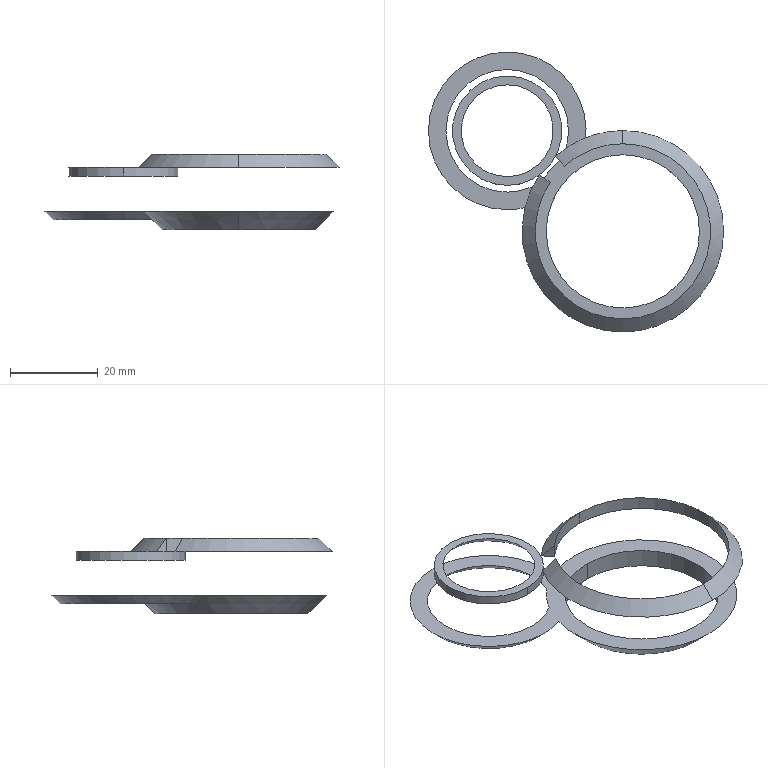Part | SolidWorks | features BaseBody 3 | 3 solids | 25 faces | box 67.409 x 63.969 x 17.243 mm | volume 2142 mm3 | cone 13 | cylinder 7 | plane 5 | commonest cylinder face diameters 40 x3 25 x2 35 x2
STEP:
#1=CARTESIAN_POINT('',(128.912,61.709,-226.962));
#2=VERTEX_POINT('',#1);
#3=CARTESIAN_POINT('',(128.912,96.709,-226.962));
#4=VERTEX_POINT('',#3);
#5=CARTESIAN_POINT('',(128.912,79.209,-226.962));
#6=DIRECTION('',(0.,0.,-1.));
#7=DIRECTION('',(0.,1.,0.));
#8=AXIS2_PLACEMENT_3D('',#5,#6,#7);
#9=CIRCLE('',#8,17.5);
#10=EDGE_CURVE('',#2,#4,#9,.T.);
#11=ORIENTED_EDGE('',*,*,#10,.F.);
#12=CARTESIAN_POINT('',(128.912,61.709,-231.204));
#13=VERTEX_POINT('',#12);
#14=CARTESIAN_POINT('',(128.912,61.709,-232.962));
#15=DIRECTION('',(0.,0.,-1.));
#16=VECTOR('',#15,1000.);
#17=LINE('',#14,#16);
#18=EDGE_CURVE('',#2,#13,#17,.T.);
#19=ORIENTED_EDGE('',*,*,#18,.T.);
#20=CARTESIAN_POINT('',(128.912,96.709,-231.204));
#21=VERTEX_POINT('',#20);
#22=CARTESIAN_POINT('',(128.912,79.209,-231.204));
#23=DIRECTION('',(0.,0.,1.));
#24=DIRECTION('',(0.,1.,0.));
#25=AXIS2_PLACEMENT_3D('',#22,#23,#24);
#26=CIRCLE('',#25,17.5);
#27=EDGE_CURVE('',#21,#13,#26,.T.);
#28=ORIENTED_EDGE('',*,*,#27,.F.);
#29=CARTESIAN_POINT('',(128.912,96.709,-232.962));
#30=DIRECTION('',(0.,0.,-1.));
#31=VECTOR('',#30,1000.);
#32=LINE('',#29,#31);
#33=EDGE_CURVE('',#4,#21,#32,.T.);
#34=ORIENTED_EDGE('',*,*,#33,.F.);
#35=EDGE_LOOP('',(#11,#19,#28,#34));
#36=FACE_OUTER_BOUND('',#35,.T.);
#37=CARTESIAN_POINT('',(128.912,79.209,-232.962));
#38=DIRECTION('',(0.,0.,-1.));
#39=DIRECTION('',(0.,1.,0.));
#40=AXIS2_PLACEMENT_3D('',#37,#38,#39);
#41=CYLINDRICAL_SURFACE('',#40,17.5);
#42=ADVANCED_FACE('',(#36),#41,.F.);
#43=CARTESIAN_POINT('',(102.503,88.178,-226.962));
#44=VERTEX_POINT('',#43);
#45=CARTESIAN_POINT('',(102.503,116.178,-226.962));
#46=VERTEX_POINT('',#45);
#47=CARTESIAN_POINT('',(102.503,102.178,-226.962));
#48=DIRECTION('',(0.,0.,-1.));
#49=DIRECTION('',(0.,1.,0.));
#50=AXIS2_PLACEMENT_3D('',#47,#48,#49);
#51=CIRCLE('',#50,14.);
#52=EDGE_CURVE('',#44,#46,#51,.T.);
#53=ORIENTED_EDGE('',*,*,#52,.F.);
#54=CARTESIAN_POINT('',(102.503,86.178,-228.962));
#55=VERTEX_POINT('',#54);
#56=CARTESIAN_POINT('',(102.503,86.178,-228.962));
#57=DIRECTION('',(0.,-0.7071,-0.7071));
#58=VECTOR('',#57,1000.);
#59=LINE('',#56,#58);
#60=EDGE_CURVE('',#44,#55,#59,.T.);
#61=ORIENTED_EDGE('',*,*,#60,.T.);
#62=CARTESIAN_POINT('',(102.503,118.178,-228.962));
#63=VERTEX_POINT('',#62);
#64=CARTESIAN_POINT('',(102.503,102.178,-228.962));
#65=DIRECTION('',(0.,0.,1.));
#66=DIRECTION('',(0.7855,0.6189,0.));
#67=AXIS2_PLACEMENT_3D('',#64,#65,#66);
#68=CIRCLE('',#67,16.);
#69=EDGE_CURVE('',#63,#55,#68,.T.);
#70=ORIENTED_EDGE('',*,*,#69,.F.);
#71=CARTESIAN_POINT('',(102.503,118.178,-228.962));
#72=DIRECTION('',(0.,0.7071,-0.7071));
#73=VECTOR('',#72,1000.);
#74=LINE('',#71,#73);
#75=EDGE_CURVE('',#46,#63,#74,.T.);
#76=ORIENTED_EDGE('',*,*,#75,.F.);
#77=EDGE_LOOP('',(#53,#61,#70,#76));
#78=FACE_OUTER_BOUND('',#77,.T.);
#79=CARTESIAN_POINT('',(102.503,102.178,-228.962));
#80=DIRECTION('',(0.,0.,-1.));
#81=DIRECTION('',(0.,1.,0.));
#82=AXIS2_PLACEMENT_3D('',#79,#80,#81);
#83=CONICAL_SURFACE('',#82,16.,0.7854);
#84=ADVANCED_FACE('',(#78),#83,.F.);
#85=CARTESIAN_POINT('',(115.043,95.955,-226.962));
#86=VERTEX_POINT('',#85);
#87=CARTESIAN_POINT('',(102.503,102.178,-226.962));
#88=DIRECTION('',(0.,0.,-1.));
#89=DIRECTION('',(0.,1.,0.));
#90=AXIS2_PLACEMENT_3D('',#87,#88,#89);
#91=CIRCLE('',#90,14.);
#92=EDGE_CURVE('',#46,#86,#91,.T.);
#93=ORIENTED_EDGE('',*,*,#92,.F.);
#94=ORIENTED_EDGE('',*,*,#75,.T.);
#95=CARTESIAN_POINT('',(116.63,94.667,-228.962));
#96=VERTEX_POINT('',#95);
#97=CARTESIAN_POINT('',(102.503,102.178,-228.962));
#98=DIRECTION('',(0.,0.,1.));
#99=DIRECTION('',(0.7855,0.6189,0.));
#100=AXIS2_PLACEMENT_3D('',#97,#98,#99);
#101=CIRCLE('',#100,16.);
#102=EDGE_CURVE('',#96,#63,#101,.T.);
#103=ORIENTED_EDGE('',*,*,#102,.F.);
#104=CARTESIAN_POINT('',(115.043,95.955,-226.962));
#105=CARTESIAN_POINT('',(115.578,95.532,-227.628));
#106=CARTESIAN_POINT('',(116.106,95.102,-228.295));
#107=CARTESIAN_POINT('',(116.63,94.667,-228.962));
#108=B_SPLINE_CURVE_WITH_KNOTS('',3,(#104,#105,#106,#107),.UNSPECIFIED.,.F.,.F.,(4,4),(0.,0.002859),.UNSPECIFIED.);
#109=EDGE_CURVE('',#86,#96,#108,.T.);
#110=ORIENTED_EDGE('',*,*,#109,.F.);
#111=EDGE_LOOP('',(#93,#94,#103,#110));
#112=FACE_OUTER_BOUND('',#111,.T.);
#113=CARTESIAN_POINT('',(102.503,102.178,-228.962));
#114=DIRECTION('',(0.,0.,-1.));
#115=DIRECTION('',(0.,1.,0.));
#116=AXIS2_PLACEMENT_3D('',#113,#114,#115);
#117=CONICAL_SURFACE('',#116,16.,0.7854);
#118=ADVANCED_FACE('',(#112),#117,.F.);
#119=CARTESIAN_POINT('',(128.912,79.209,-231.204));
#120=DIRECTION('',(0.,0.,1.));
#121=DIRECTION('',(0.,1.,0.));
#122=AXIS2_PLACEMENT_3D('',#119,#120,#121);
#123=CIRCLE('',#122,17.5);
#124=EDGE_CURVE('',#13,#21,#123,.T.);
#125=ORIENTED_EDGE('',*,*,#124,.T.);
#126=CARTESIAN_POINT('',(128.912,100.952,-226.962));
#127=VERTEX_POINT('',#126);
#128=CARTESIAN_POINT('',(128.912,100.952,-226.962));
#129=DIRECTION('',(0.,0.7071,0.7071));
#130=VECTOR('',#129,1000.);
#131=LINE('',#128,#130);
#132=EDGE_CURVE('',#21,#127,#131,.T.);
#133=ORIENTED_EDGE('',*,*,#132,.T.);
#134=CARTESIAN_POINT('',(128.912,57.467,-226.962));
#135=VERTEX_POINT('',#134);
#136=CARTESIAN_POINT('',(128.912,79.209,-226.962));
#137=DIRECTION('',(0.,0.,1.));
#138=DIRECTION('',(0.,-1.,0.));
#139=AXIS2_PLACEMENT_3D('',#136,#137,#138);
#140=CIRCLE('',#139,21.743);
#141=EDGE_CURVE('',#135,#127,#140,.T.);
#142=ORIENTED_EDGE('',*,*,#141,.F.);
#143=CARTESIAN_POINT('',(128.912,57.467,-226.962));
#144=DIRECTION('',(0.,-0.7071,0.7071));
#145=VECTOR('',#144,1000.);
#146=LINE('',#143,#145);
#147=EDGE_CURVE('',#13,#135,#146,.T.);
#148=ORIENTED_EDGE('',*,*,#147,.F.);
#149=EDGE_LOOP('',(#125,#133,#142,#148));
#150=FACE_OUTER_BOUND('',#149,.T.);
#151=CARTESIAN_POINT('',(128.912,79.209,-226.962));
#152=DIRECTION('',(0.,0.,1.));
#153=DIRECTION('',(0.,-1.,0.));
#154=AXIS2_PLACEMENT_3D('',#151,#152,#153);
#155=CONICAL_SURFACE('',#154,21.743,0.7854);
#156=ADVANCED_FACE('',(#150),#155,.T.);
#157=ORIENTED_EDGE('',*,*,#102,.T.);
#158=CARTESIAN_POINT('',(102.503,120.178,-226.962));
#159=VERTEX_POINT('',#158);
#160=CARTESIAN_POINT('',(102.503,120.178,-226.962));
#161=DIRECTION('',(0.,0.7071,0.7071));
#162=VECTOR('',#161,1000.);
#163=LINE('',#160,#162);
#164=EDGE_CURVE('',#63,#159,#163,.T.);
#165=ORIENTED_EDGE('',*,*,#164,.T.);
#166=CARTESIAN_POINT('',(120.246,99.151,-226.962));
#167=VERTEX_POINT('',#166);
#168=CARTESIAN_POINT('',(102.503,102.178,-226.962));
#169=DIRECTION('',(0.,0.,1.));
#170=DIRECTION('',(0.,-1.,0.));
#171=AXIS2_PLACEMENT_3D('',#168,#169,#170);
#172=CIRCLE('',#171,18.);
#173=EDGE_CURVE('',#167,#159,#172,.T.);
#174=ORIENTED_EDGE('',*,*,#173,.F.);
#175=CARTESIAN_POINT('',(116.63,94.667,-228.962));
#176=CARTESIAN_POINT('',(117.273,95.439,-228.757));
#177=CARTESIAN_POINT('',(117.891,96.196,-228.476));
#178=CARTESIAN_POINT('',(119.093,97.689,-227.798));
#179=CARTESIAN_POINT('',(119.676,98.424,-227.401));
#180=CARTESIAN_POINT('',(120.246,99.151,-226.962));
#181=B_SPLINE_CURVE_WITH_KNOTS('',3,(#175,#176,#177,#178,#179,#180),.UNSPECIFIED.,.F.,.F.,(4,2,4),(0.,0.003049,0.006098),.UNSPECIFIED.);
#182=EDGE_CURVE('',#96,#167,#181,.T.);
#183=ORIENTED_EDGE('',*,*,#182,.F.);
#184=EDGE_LOOP('',(#157,#165,#174,#183));
#185=FACE_OUTER_BOUND('',#184,.T.);
#186=CARTESIAN_POINT('',(102.503,102.178,-226.962));
#187=DIRECTION('',(0.,0.,1.));
#188=DIRECTION('',(0.,-1.,0.));
#189=AXIS2_PLACEMENT_3D('',#186,#187,#188);
#190=CONICAL_SURFACE('',#189,18.,0.7854);
#191=ADVANCED_FACE('',(#185),#190,.T.);
#192=ORIENTED_EDGE('',*,*,#164,.F.);
#193=ORIENTED_EDGE('',*,*,#69,.T.);
#194=CARTESIAN_POINT('',(102.503,84.178,-226.962));
#195=VERTEX_POINT('',#194);
#196=CARTESIAN_POINT('',(102.503,84.178,-226.962));
#197=DIRECTION('',(0.,-0.7071,0.7071));
#198=VECTOR('',#197,1000.);
#199=LINE('',#196,#198);
#200=EDGE_CURVE('',#55,#195,#199,.T.);
#201=ORIENTED_EDGE('',*,*,#200,.T.);
#202=CARTESIAN_POINT('',(102.503,102.178,-226.962));
#203=DIRECTION('',(0.,0.,1.));
#204=DIRECTION('',(0.,-1.,0.));
#205=AXIS2_PLACEMENT_3D('',#202,#203,#204);
#206=CIRCLE('',#205,18.);
#207=EDGE_CURVE('',#159,#195,#206,.T.);
#208=ORIENTED_EDGE('',*,*,#207,.F.);
#209=EDGE_LOOP('',(#192,#193,#201,#208));
#210=FACE_OUTER_BOUND('',#209,.T.);
#211=CARTESIAN_POINT('',(102.503,102.178,-226.962));
#212=DIRECTION('',(0.,0.,1.));
#213=DIRECTION('',(0.,-1.,0.));
#214=AXIS2_PLACEMENT_3D('',#211,#212,#213);
#215=CONICAL_SURFACE('',#214,18.,0.7854);
#216=ADVANCED_FACE('',(#210),#215,.T.);
#217=CARTESIAN_POINT('',(128.912,79.209,-226.962));
#218=DIRECTION('',(0.,0.,-1.));
#219=DIRECTION('',(0.,1.,0.));
#220=AXIS2_PLACEMENT_3D('',#217,#218,#219);
#221=CIRCLE('',#220,17.5);
#222=EDGE_CURVE('',#4,#2,#221,.T.);
#223=ORIENTED_EDGE('',*,*,#222,.T.);
#224=ORIENTED_EDGE('',*,*,#10,.T.);
#225=EDGE_LOOP('',(#223,#224));
#226=FACE_BOUND('',#225,.T.);
#227=CARTESIAN_POINT('',(110.405,90.621,-226.962));
#228=VERTEX_POINT('',#227);
#229=CARTESIAN_POINT('',(128.912,79.209,-226.962));
#230=DIRECTION('',(0.,0.,1.));
#231=DIRECTION('',(0.,-1.,0.));
#232=AXIS2_PLACEMENT_3D('',#229,#230,#231);
#233=CIRCLE('',#232,21.743);
#234=EDGE_CURVE('',#86,#228,#233,.T.);
#235=ORIENTED_EDGE('',*,*,#234,.T.);
#236=CARTESIAN_POINT('',(102.503,102.178,-226.962));
#237=DIRECTION('',(0.,0.,-1.));
#238=DIRECTION('',(0.,1.,0.));
#239=AXIS2_PLACEMENT_3D('',#236,#237,#238);
#240=CIRCLE('',#239,14.);
#241=EDGE_CURVE('',#228,#44,#240,.T.);
#242=ORIENTED_EDGE('',*,*,#241,.T.);
#243=ORIENTED_EDGE('',*,*,#52,.T.);
#244=ORIENTED_EDGE('',*,*,#92,.T.);
#245=EDGE_LOOP('',(#235,#242,#243,#244));
#246=FACE_BOUND('',#245,.T.);
#247=ORIENTED_EDGE('',*,*,#173,.T.);
#248=ORIENTED_EDGE('',*,*,#207,.T.);
#249=CARTESIAN_POINT('',(107.961,85.026,-226.962));
#250=VERTEX_POINT('',#249);
#251=CARTESIAN_POINT('',(102.503,102.178,-226.962));
#252=DIRECTION('',(0.,0.,1.));
#253=DIRECTION('',(0.,-1.,0.));
#254=AXIS2_PLACEMENT_3D('',#251,#252,#253);
#255=CIRCLE('',#254,18.);
#256=EDGE_CURVE('',#195,#250,#255,.T.);
#257=ORIENTED_EDGE('',*,*,#256,.T.);
#258=CARTESIAN_POINT('',(128.912,79.209,-226.962));
#259=DIRECTION('',(0.,0.,1.));
#260=DIRECTION('',(0.,-1.,0.));
#261=AXIS2_PLACEMENT_3D('',#258,#259,#260);
#262=CIRCLE('',#261,21.743);
#263=EDGE_CURVE('',#250,#135,#262,.T.);
#264=ORIENTED_EDGE('',*,*,#263,.T.);
#265=ORIENTED_EDGE('',*,*,#141,.T.);
#266=CARTESIAN_POINT('',(128.912,79.209,-226.962));
#267=DIRECTION('',(0.,0.,1.));
#268=DIRECTION('',(0.,-1.,0.));
#269=AXIS2_PLACEMENT_3D('',#266,#267,#268);
#270=CIRCLE('',#269,21.743);
#271=EDGE_CURVE('',#127,#167,#270,.T.);
#272=ORIENTED_EDGE('',*,*,#271,.T.);
#273=EDGE_LOOP('',(#247,#248,#257,#264,#265,#272));
#274=FACE_OUTER_BOUND('',#273,.T.);
#275=CARTESIAN_POINT('',(115.707,90.694,-226.962));
#276=DIRECTION('',(0.,0.,1.));
#277=DIRECTION('',(0.,-1.,0.));
#278=AXIS2_PLACEMENT_3D('',#275,#276,#277);
#279=PLANE('',#278);
#280=ADVANCED_FACE('',(#226,#246,#274),#279,.T.);
#281=ORIENTED_EDGE('',*,*,#18,.F.);
#282=ORIENTED_EDGE('',*,*,#222,.F.);
#283=ORIENTED_EDGE('',*,*,#33,.T.);
#284=ORIENTED_EDGE('',*,*,#124,.F.);
#285=EDGE_LOOP('',(#281,#282,#283,#284));
#286=FACE_OUTER_BOUND('',#285,.T.);
#287=CARTESIAN_POINT('',(128.912,79.209,-232.962));
#288=DIRECTION('',(0.,0.,-1.));
#289=DIRECTION('',(0.,1.,0.));
#290=AXIS2_PLACEMENT_3D('',#287,#288,#289);
#291=CYLINDRICAL_SURFACE('',#290,17.5);
#292=ADVANCED_FACE('',(#286),#291,.F.);
#293=ORIENTED_EDGE('',*,*,#60,.F.);
#294=ORIENTED_EDGE('',*,*,#241,.F.);
#295=CARTESIAN_POINT('',(111.901,89.229,-228.962));
#296=VERTEX_POINT('',#295);
#297=CARTESIAN_POINT('',(111.901,89.229,-228.962));
#298=CARTESIAN_POINT('',(111.396,89.687,-228.295));
#299=CARTESIAN_POINT('',(110.898,90.151,-227.628));
#300=CARTESIAN_POINT('',(110.405,90.621,-226.962));
#301=B_SPLINE_CURVE_WITH_KNOTS('',3,(#297,#298,#299,#300),.UNSPECIFIED.,.F.,.F.,(4,4),(0.,0.002859),.UNSPECIFIED.);
#302=EDGE_CURVE('',#296,#228,#301,.T.);
#303=ORIENTED_EDGE('',*,*,#302,.F.);
#304=CARTESIAN_POINT('',(102.503,102.178,-228.962));
#305=DIRECTION('',(0.,0.,1.));
#306=DIRECTION('',(0.7855,0.6189,0.));
#307=AXIS2_PLACEMENT_3D('',#304,#305,#306);
#308=CIRCLE('',#307,16.);
#309=EDGE_CURVE('',#55,#296,#308,.T.);
#310=ORIENTED_EDGE('',*,*,#309,.F.);
#311=EDGE_LOOP('',(#293,#294,#303,#310));
#312=FACE_OUTER_BOUND('',#311,.T.);
#313=CARTESIAN_POINT('',(102.503,102.178,-228.962));
#314=DIRECTION('',(0.,0.,-1.));
#315=DIRECTION('',(0.,1.,0.));
#316=AXIS2_PLACEMENT_3D('',#313,#314,#315);
#317=CONICAL_SURFACE('',#316,16.,0.7854);
#318=ADVANCED_FACE('',(#312),#317,.F.);
#319=ORIENTED_EDGE('',*,*,#132,.F.);
#320=ORIENTED_EDGE('',*,*,#27,.T.);
#321=ORIENTED_EDGE('',*,*,#147,.T.);
#322=ORIENTED_EDGE('',*,*,#263,.F.);
#323=CARTESIAN_POINT('',(107.961,85.026,-226.962));
#324=CARTESIAN_POINT('',(108.602,85.691,-227.401));
#325=CARTESIAN_POINT('',(109.249,86.37,-227.798));
#326=CARTESIAN_POINT('',(110.56,87.767,-228.476));
#327=CARTESIAN_POINT('',(111.225,88.485,-228.757));
#328=CARTESIAN_POINT('',(111.901,89.229,-228.962));
#329=B_SPLINE_CURVE_WITH_KNOTS('',3,(#323,#324,#325,#326,#327,#328),.UNSPECIFIED.,.F.,.F.,(4,2,4),(0.,0.003049,0.006098),.UNSPECIFIED.);
#330=EDGE_CURVE('',#250,#296,#329,.T.);
#331=ORIENTED_EDGE('',*,*,#330,.T.);
#332=ORIENTED_EDGE('',*,*,#302,.T.);
#333=ORIENTED_EDGE('',*,*,#234,.F.);
#334=ORIENTED_EDGE('',*,*,#109,.T.);
#335=ORIENTED_EDGE('',*,*,#182,.T.);
#336=ORIENTED_EDGE('',*,*,#271,.F.);
#337=EDGE_LOOP('',(#319,#320,#321,#322,#331,#332,#333,#334,#335,#336));
#338=FACE_OUTER_BOUND('',#337,.T.);
#339=CARTESIAN_POINT('',(128.912,79.209,-226.962));
#340=DIRECTION('',(0.,0.,1.));
#341=DIRECTION('',(0.,-1.,0.));
#342=AXIS2_PLACEMENT_3D('',#339,#340,#341);
#343=CONICAL_SURFACE('',#342,21.743,0.7854);
#344=ADVANCED_FACE('',(#338),#343,.T.);
#345=ORIENTED_EDGE('',*,*,#200,.F.);
#346=ORIENTED_EDGE('',*,*,#309,.T.);
#347=ORIENTED_EDGE('',*,*,#330,.F.);
#348=ORIENTED_EDGE('',*,*,#256,.F.);
#349=EDGE_LOOP('',(#345,#346,#347,#348));
#350=FACE_OUTER_BOUND('',#349,.T.);
#351=CARTESIAN_POINT('',(102.503,102.178,-226.962));
#352=DIRECTION('',(0.,0.,1.));
#353=DIRECTION('',(0.,-1.,0.));
#354=AXIS2_PLACEMENT_3D('',#351,#352,#353);
#355=CONICAL_SURFACE('',#354,18.,0.7854);
#356=ADVANCED_FACE('',(#350),#355,.T.);
#357=CLOSED_SHELL('',(#42,#84,#118,#156,#191,#216,#280,#292,#318,#344,#356));
#358=MANIFOLD_SOLID_BREP('',#357);
#359=CARTESIAN_POINT('',(102.503,91.678,-216.962));
#360=VERTEX_POINT('',#359);
#361=CARTESIAN_POINT('',(102.503,112.678,-216.962));
#362=VERTEX_POINT('',#361);
#363=CARTESIAN_POINT('',(102.503,102.178,-216.962));
#364=DIRECTION('',(0.,0.,-1.));
#365=DIRECTION('',(0.,1.,0.));
#366=AXIS2_PLACEMENT_3D('',#363,#364,#365);
#367=CIRCLE('',#366,10.5);
#368=EDGE_CURVE('',#360,#362,#367,.T.);
#369=ORIENTED_EDGE('',*,*,#368,.F.);
#370=CARTESIAN_POINT('',(102.503,89.678,-218.962));
#371=VERTEX_POINT('',#370);
#372=CARTESIAN_POINT('',(102.503,89.678,-218.962));
#373=DIRECTION('',(0.,-0.7071,-0.7071));
#374=VECTOR('',#373,1000.);
#375=LINE('',#372,#374);
#376=EDGE_CURVE('',#360,#371,#375,.T.);
#377=ORIENTED_EDGE('',*,*,#376,.T.);
#378=CARTESIAN_POINT('',(102.503,114.678,-218.962));
#379=VERTEX_POINT('',#378);
#380=CARTESIAN_POINT('',(102.503,102.178,-218.962));
#381=DIRECTION('',(0.,0.,1.));
#382=DIRECTION('',(0.7855,0.6189,0.));
#383=AXIS2_PLACEMENT_3D('',#380,#381,#382);
#384=CIRCLE('',#383,12.5);
#385=EDGE_CURVE('',#379,#371,#384,.T.);
#386=ORIENTED_EDGE('',*,*,#385,.F.);
#387=CARTESIAN_POINT('',(102.503,114.678,-218.962));
#388=DIRECTION('',(0.,0.7071,-0.7071));
#389=VECTOR('',#388,1000.);
#390=LINE('',#387,#389);
#391=EDGE_CURVE('',#362,#379,#390,.T.);
#392=ORIENTED_EDGE('',*,*,#391,.F.);
#393=EDGE_LOOP('',(#369,#377,#386,#392));
#394=FACE_OUTER_BOUND('',#393,.T.);
#395=CARTESIAN_POINT('',(102.503,102.178,-218.962));
#396=DIRECTION('',(0.,0.,-1.));
#397=DIRECTION('',(0.,1.,0.));
#398=AXIS2_PLACEMENT_3D('',#395,#396,#397);
#399=CONICAL_SURFACE('',#398,12.5,0.7854);
#400=ADVANCED_FACE('',(#394),#399,.F.);
#401=CARTESIAN_POINT('',(102.503,102.178,-218.962));
#402=DIRECTION('',(0.,0.,1.));
#403=DIRECTION('',(0.7855,0.6189,0.));
#404=AXIS2_PLACEMENT_3D('',#401,#402,#403);
#405=CIRCLE('',#404,12.5);
#406=EDGE_CURVE('',#371,#379,#405,.T.);
#407=ORIENTED_EDGE('',*,*,#406,.T.);
#408=CARTESIAN_POINT('',(102.503,114.678,-216.962));
#409=VERTEX_POINT('',#408);
#410=CARTESIAN_POINT('',(102.503,114.678,-226.962));
#411=DIRECTION('',(0.,0.,1.));
#412=VECTOR('',#411,1000.);
#413=LINE('',#410,#412);
#414=EDGE_CURVE('',#379,#409,#413,.T.);
#415=ORIENTED_EDGE('',*,*,#414,.T.);
#416=CARTESIAN_POINT('',(102.503,89.678,-216.962));
#417=VERTEX_POINT('',#416);
#418=CARTESIAN_POINT('',(102.503,102.178,-216.962));
#419=DIRECTION('',(0.,0.,-1.));
#420=DIRECTION('',(0.,-1.,0.));
#421=AXIS2_PLACEMENT_3D('',#418,#419,#420);
#422=CIRCLE('',#421,12.5);
#423=EDGE_CURVE('',#409,#417,#422,.T.);
#424=ORIENTED_EDGE('',*,*,#423,.T.);
#425=CARTESIAN_POINT('',(102.503,89.678,-226.962));
#426=DIRECTION('',(0.,0.,1.));
#427=VECTOR('',#426,1000.);
#428=LINE('',#425,#427);
#429=EDGE_CURVE('',#371,#417,#428,.T.);
#430=ORIENTED_EDGE('',*,*,#429,.F.);
#431=EDGE_LOOP('',(#407,#415,#424,#430));
#432=FACE_OUTER_BOUND('',#431,.T.);
#433=CARTESIAN_POINT('',(102.503,102.178,-226.962));
#434=DIRECTION('',(0.,0.,1.));
#435=DIRECTION('',(0.,-1.,0.));
#436=AXIS2_PLACEMENT_3D('',#433,#434,#435);
#437=CYLINDRICAL_SURFACE('',#436,12.5);
#438=ADVANCED_FACE('',(#432),#437,.T.);
#439=ORIENTED_EDGE('',*,*,#376,.F.);
#440=CARTESIAN_POINT('',(102.503,102.178,-216.962));
#441=DIRECTION('',(0.,0.,-1.));
#442=DIRECTION('',(0.,1.,0.));
#443=AXIS2_PLACEMENT_3D('',#440,#441,#442);
#444=CIRCLE('',#443,10.5);
#445=EDGE_CURVE('',#362,#360,#444,.T.);
#446=ORIENTED_EDGE('',*,*,#445,.F.);
#447=ORIENTED_EDGE('',*,*,#391,.T.);
#448=ORIENTED_EDGE('',*,*,#406,.F.);
#449=EDGE_LOOP('',(#439,#446,#447,#448));
#450=FACE_OUTER_BOUND('',#449,.T.);
#451=CARTESIAN_POINT('',(102.503,102.178,-218.962));
#452=DIRECTION('',(0.,0.,-1.));
#453=DIRECTION('',(0.,1.,0.));
#454=AXIS2_PLACEMENT_3D('',#451,#452,#453);
#455=CONICAL_SURFACE('',#454,12.5,0.7854);
#456=ADVANCED_FACE('',(#450),#455,.F.);
#457=ORIENTED_EDGE('',*,*,#414,.F.);
#458=ORIENTED_EDGE('',*,*,#385,.T.);
#459=ORIENTED_EDGE('',*,*,#429,.T.);
#460=CARTESIAN_POINT('',(102.503,102.178,-216.962));
#461=DIRECTION('',(0.,0.,-1.));
#462=DIRECTION('',(0.,-1.,0.));
#463=AXIS2_PLACEMENT_3D('',#460,#461,#462);
#464=CIRCLE('',#463,12.5);
#465=EDGE_CURVE('',#417,#409,#464,.T.);
#466=ORIENTED_EDGE('',*,*,#465,.T.);
#467=EDGE_LOOP('',(#457,#458,#459,#466));
#468=FACE_OUTER_BOUND('',#467,.T.);
#469=CARTESIAN_POINT('',(102.503,102.178,-226.962));
#470=DIRECTION('',(0.,0.,1.));
#471=DIRECTION('',(0.,-1.,0.));
#472=AXIS2_PLACEMENT_3D('',#469,#470,#471);
#473=CYLINDRICAL_SURFACE('',#472,12.5);
#474=ADVANCED_FACE('',(#468),#473,.T.);
#475=ORIENTED_EDGE('',*,*,#445,.T.);
#476=ORIENTED_EDGE('',*,*,#368,.T.);
#477=EDGE_LOOP('',(#475,#476));
#478=FACE_BOUND('',#477,.T.);
#479=ORIENTED_EDGE('',*,*,#465,.F.);
#480=ORIENTED_EDGE('',*,*,#423,.F.);
#481=EDGE_LOOP('',(#479,#480));
#482=FACE_OUTER_BOUND('',#481,.T.);
#483=CARTESIAN_POINT('',(93.071,110.381,-216.962));
#484=DIRECTION('',(0.,0.,-1.));
#485=DIRECTION('',(0.,1.,0.));
#486=AXIS2_PLACEMENT_3D('',#483,#484,#485);
#487=PLANE('',#486);
#488=ADVANCED_FACE('',(#478,#482),#487,.F.);
#489=CLOSED_SHELL('',(#400,#438,#456,#474,#488));
#490=MANIFOLD_SOLID_BREP('',#489);
#491=CARTESIAN_POINT('',(128.912,99.209,-213.962));
#492=VERTEX_POINT('',#491);
#493=CARTESIAN_POINT('',(128.912,59.209,-213.962));
#494=VERTEX_POINT('',#493);
#495=CARTESIAN_POINT('',(128.912,79.209,-213.962));
#496=DIRECTION('',(0.,0.,-1.));
#497=DIRECTION('',(0.7545,-0.6562,0.));
#498=AXIS2_PLACEMENT_3D('',#495,#496,#497);
#499=CIRCLE('',#498,20.);
#500=EDGE_CURVE('',#492,#494,#499,.T.);
#501=ORIENTED_EDGE('',*,*,#500,.T.);
#502=CARTESIAN_POINT('',(128.912,56.209,-216.962));
#503=VERTEX_POINT('',#502);
#504=CARTESIAN_POINT('',(128.912,56.209,-216.962));
#505=DIRECTION('',(0.,-0.7071,-0.7071));
#506=VECTOR('',#505,1000.);
#507=LINE('',#504,#506);
#508=EDGE_CURVE('',#494,#503,#507,.T.);
#509=ORIENTED_EDGE('',*,*,#508,.T.);
#510=CARTESIAN_POINT('',(128.912,102.209,-216.962));
#511=VERTEX_POINT('',#510);
#512=CARTESIAN_POINT('',(128.912,79.209,-216.962));
#513=DIRECTION('',(0.,0.,1.));
#514=DIRECTION('',(0.,1.,0.));
#515=AXIS2_PLACEMENT_3D('',#512,#513,#514);
#516=CIRCLE('',#515,23.);
#517=EDGE_CURVE('',#503,#511,#516,.T.);
#518=ORIENTED_EDGE('',*,*,#517,.T.);
#519=CARTESIAN_POINT('',(128.912,102.209,-216.962));
#520=DIRECTION('',(0.,0.7071,-0.7071));
#521=VECTOR('',#520,1000.);
#522=LINE('',#519,#521);
#523=EDGE_CURVE('',#492,#511,#522,.T.);
#524=ORIENTED_EDGE('',*,*,#523,.F.);
#525=EDGE_LOOP('',(#501,#509,#518,#524));
#526=FACE_OUTER_BOUND('',#525,.T.);
#527=CARTESIAN_POINT('',(128.912,79.209,-216.962));
#528=DIRECTION('',(0.,0.,-1.));
#529=DIRECTION('',(0.,1.,0.));
#530=AXIS2_PLACEMENT_3D('',#527,#528,#529);
#531=CONICAL_SURFACE('',#530,23.,0.7854);
#532=ADVANCED_FACE('',(#526),#531,.T.);
#533=CARTESIAN_POINT('',(115.552,94.092,-213.962));
#534=VERTEX_POINT('',#533);
#535=CARTESIAN_POINT('',(128.912,79.209,-213.962));
#536=DIRECTION('',(0.,0.,-1.));
#537=DIRECTION('',(0.7545,-0.6562,0.));
#538=AXIS2_PLACEMENT_3D('',#535,#536,#537);
#539=CIRCLE('',#538,20.);
#540=EDGE_CURVE('',#534,#492,#539,.T.);
#541=ORIENTED_EDGE('',*,*,#540,.T.);
#542=ORIENTED_EDGE('',*,*,#523,.T.);
#543=CARTESIAN_POINT('',(113.548,96.325,-216.962));
#544=VERTEX_POINT('',#543);
#545=CARTESIAN_POINT('',(128.912,79.209,-216.962));
#546=DIRECTION('',(0.,0.,1.));
#547=DIRECTION('',(0.,1.,0.));
#548=AXIS2_PLACEMENT_3D('',#545,#546,#547);
#549=CIRCLE('',#548,23.);
#550=EDGE_CURVE('',#511,#544,#549,.T.);
#551=ORIENTED_EDGE('',*,*,#550,.T.);
#552=CARTESIAN_POINT('',(113.548,96.325,-216.962));
#553=DIRECTION('',(0.4724,-0.5262,0.7071));
#554=VECTOR('',#553,1000.);
#555=LINE('',#552,#554);
#556=EDGE_CURVE('',#544,#534,#555,.T.);
#557=ORIENTED_EDGE('',*,*,#556,.T.);
#558=EDGE_LOOP('',(#541,#542,#551,#557));
#559=FACE_OUTER_BOUND('',#558,.T.);
#560=CARTESIAN_POINT('',(128.912,79.209,-216.962));
#561=DIRECTION('',(0.,0.,-1.));
#562=DIRECTION('',(0.,1.,0.));
#563=AXIS2_PLACEMENT_3D('',#560,#561,#562);
#564=CONICAL_SURFACE('',#563,23.,0.7854);
#565=ADVANCED_FACE('',(#559),#564,.T.);
#566=CARTESIAN_POINT('',(112.32,90.376,-213.962));
#567=VERTEX_POINT('',#566);
#568=CARTESIAN_POINT('',(128.912,79.209,-213.962));
#569=DIRECTION('',(0.,0.,-1.));
#570=DIRECTION('',(0.7545,-0.6562,0.));
#571=AXIS2_PLACEMENT_3D('',#568,#569,#570);
#572=CIRCLE('',#571,20.);
#573=EDGE_CURVE('',#494,#567,#572,.T.);
#574=ORIENTED_EDGE('',*,*,#573,.F.);
#575=CARTESIAN_POINT('',(128.912,59.209,-216.962));
#576=VERTEX_POINT('',#575);
#577=CARTESIAN_POINT('',(128.912,59.209,-215.462));
#578=DIRECTION('',(0.,0.,-1.));
#579=VECTOR('',#578,1000.);
#580=LINE('',#577,#579);
#581=EDGE_CURVE('',#494,#576,#580,.T.);
#582=ORIENTED_EDGE('',*,*,#581,.T.);
#583=CARTESIAN_POINT('',(112.32,90.376,-216.962));
#584=VERTEX_POINT('',#583);
#585=CARTESIAN_POINT('',(128.912,79.209,-216.962));
#586=DIRECTION('',(0.,0.,1.));
#587=DIRECTION('',(0.,1.,0.));
#588=AXIS2_PLACEMENT_3D('',#585,#586,#587);
#589=CIRCLE('',#588,20.);
#590=EDGE_CURVE('',#584,#576,#589,.T.);
#591=ORIENTED_EDGE('',*,*,#590,.F.);
#592=CARTESIAN_POINT('',(112.32,90.376,-216.962));
#593=DIRECTION('',(0.,0.,-1.));
#594=VECTOR('',#593,1000.);
#595=LINE('',#592,#594);
#596=EDGE_CURVE('',#567,#584,#595,.T.);
#597=ORIENTED_EDGE('',*,*,#596,.F.);
#598=EDGE_LOOP('',(#574,#582,#591,#597));
#599=FACE_OUTER_BOUND('',#598,.T.);
#600=CARTESIAN_POINT('',(128.912,79.209,-215.462));
#601=DIRECTION('',(0.,0.,-1.));
#602=DIRECTION('',(0.,1.,0.));
#603=AXIS2_PLACEMENT_3D('',#600,#601,#602);
#604=CYLINDRICAL_SURFACE('',#603,20.);
#605=ADVANCED_FACE('',(#599),#604,.F.);
#606=ORIENTED_EDGE('',*,*,#581,.F.);
#607=ORIENTED_EDGE('',*,*,#500,.F.);
#608=CARTESIAN_POINT('',(128.912,99.209,-216.962));
#609=VERTEX_POINT('',#608);
#610=CARTESIAN_POINT('',(128.912,99.209,-215.462));
#611=DIRECTION('',(0.,0.,-1.));
#612=VECTOR('',#611,1000.);
#613=LINE('',#610,#612);
#614=EDGE_CURVE('',#492,#609,#613,.T.);
#615=ORIENTED_EDGE('',*,*,#614,.T.);
#616=CARTESIAN_POINT('',(128.912,79.209,-216.962));
#617=DIRECTION('',(0.,0.,1.));
#618=DIRECTION('',(0.,1.,0.));
#619=AXIS2_PLACEMENT_3D('',#616,#617,#618);
#620=CIRCLE('',#619,20.);
#621=EDGE_CURVE('',#576,#609,#620,.T.);
#622=ORIENTED_EDGE('',*,*,#621,.F.);
#623=EDGE_LOOP('',(#606,#607,#615,#622));
#624=FACE_OUTER_BOUND('',#623,.T.);
#625=CARTESIAN_POINT('',(128.912,79.209,-215.462));
#626=DIRECTION('',(0.,0.,-1.));
#627=DIRECTION('',(0.,1.,0.));
#628=AXIS2_PLACEMENT_3D('',#625,#626,#627);
#629=CYLINDRICAL_SURFACE('',#628,20.);
#630=ADVANCED_FACE('',(#624),#629,.F.);
#631=ORIENTED_EDGE('',*,*,#508,.F.);
#632=ORIENTED_EDGE('',*,*,#573,.T.);
#633=CARTESIAN_POINT('',(109.831,92.051,-216.962));
#634=VERTEX_POINT('',#633);
#635=CARTESIAN_POINT('',(109.831,92.051,-216.962));
#636=DIRECTION('',(-0.5866,0.3948,-0.7071));
#637=VECTOR('',#636,1000.);
#638=LINE('',#635,#637);
#639=EDGE_CURVE('',#567,#634,#638,.T.);
#640=ORIENTED_EDGE('',*,*,#639,.T.);
#641=CARTESIAN_POINT('',(128.912,79.209,-216.962));
#642=DIRECTION('',(0.,0.,1.));
#643=DIRECTION('',(0.,1.,0.));
#644=AXIS2_PLACEMENT_3D('',#641,#642,#643);
#645=CIRCLE('',#644,23.);
#646=EDGE_CURVE('',#634,#503,#645,.T.);
#647=ORIENTED_EDGE('',*,*,#646,.T.);
#648=EDGE_LOOP('',(#631,#632,#640,#647));
#649=FACE_OUTER_BOUND('',#648,.T.);
#650=CARTESIAN_POINT('',(128.912,79.209,-216.962));
#651=DIRECTION('',(0.,0.,-1.));
#652=DIRECTION('',(0.,1.,0.));
#653=AXIS2_PLACEMENT_3D('',#650,#651,#652);
#654=CONICAL_SURFACE('',#653,23.,0.7854);
#655=ADVANCED_FACE('',(#649),#654,.T.);
#656=ORIENTED_EDGE('',*,*,#596,.T.);
#657=CARTESIAN_POINT('',(112.32,90.376,-216.962));
#658=DIRECTION('',(-0.8296,0.5584,0.));
#659=VECTOR('',#658,1000.);
#660=LINE('',#657,#659);
#661=EDGE_CURVE('',#584,#634,#660,.T.);
#662=ORIENTED_EDGE('',*,*,#661,.T.);
#663=ORIENTED_EDGE('',*,*,#639,.F.);
#664=EDGE_LOOP('',(#656,#662,#663));
#665=FACE_OUTER_BOUND('',#664,.T.);
#666=CARTESIAN_POINT('',(112.32,90.376,-216.962));
#667=DIRECTION('',(0.5584,0.8296,0.));
#668=DIRECTION('',(-0.8296,0.5584,0.));
#669=AXIS2_PLACEMENT_3D('',#666,#667,#668);
#670=PLANE('',#669);
#671=ADVANCED_FACE('',(#665),#670,.T.);
#672=ORIENTED_EDGE('',*,*,#614,.F.);
#673=ORIENTED_EDGE('',*,*,#540,.F.);
#674=CARTESIAN_POINT('',(115.552,94.092,-216.962));
#675=VERTEX_POINT('',#674);
#676=CARTESIAN_POINT('',(115.552,94.092,-215.462));
#677=DIRECTION('',(0.,0.,1.));
#678=VECTOR('',#677,1000.);
#679=LINE('',#676,#678);
#680=EDGE_CURVE('',#675,#534,#679,.T.);
#681=ORIENTED_EDGE('',*,*,#680,.F.);
#682=CARTESIAN_POINT('',(128.912,79.209,-216.962));
#683=DIRECTION('',(0.,0.,1.));
#684=DIRECTION('',(0.,1.,0.));
#685=AXIS2_PLACEMENT_3D('',#682,#683,#684);
#686=CIRCLE('',#685,20.);
#687=EDGE_CURVE('',#609,#675,#686,.T.);
#688=ORIENTED_EDGE('',*,*,#687,.F.);
#689=EDGE_LOOP('',(#672,#673,#681,#688));
#690=FACE_OUTER_BOUND('',#689,.T.);
#691=CARTESIAN_POINT('',(128.912,79.209,-215.462));
#692=DIRECTION('',(0.,0.,-1.));
#693=DIRECTION('',(0.,1.,0.));
#694=AXIS2_PLACEMENT_3D('',#691,#692,#693);
#695=CYLINDRICAL_SURFACE('',#694,20.);
#696=ADVANCED_FACE('',(#690),#695,.F.);
#697=CARTESIAN_POINT('',(115.552,94.092,-216.962));
#698=DIRECTION('',(0.668,-0.7442,0.));
#699=VECTOR('',#698,1000.);
#700=LINE('',#697,#699);
#701=EDGE_CURVE('',#544,#675,#700,.T.);
#702=ORIENTED_EDGE('',*,*,#701,.T.);
#703=ORIENTED_EDGE('',*,*,#680,.T.);
#704=ORIENTED_EDGE('',*,*,#556,.F.);
#705=EDGE_LOOP('',(#702,#703,#704));
#706=FACE_OUTER_BOUND('',#705,.T.);
#707=CARTESIAN_POINT('',(115.552,94.092,-216.962));
#708=DIRECTION('',(-0.7442,-0.668,0.));
#709=DIRECTION('',(0.668,-0.7442,0.));
#710=AXIS2_PLACEMENT_3D('',#707,#708,#709);
#711=PLANE('',#710);
#712=ADVANCED_FACE('',(#706),#711,.T.);
#713=ORIENTED_EDGE('',*,*,#646,.F.);
#714=ORIENTED_EDGE('',*,*,#661,.F.);
#715=ORIENTED_EDGE('',*,*,#590,.T.);
#716=ORIENTED_EDGE('',*,*,#621,.T.);
#717=ORIENTED_EDGE('',*,*,#687,.T.);
#718=ORIENTED_EDGE('',*,*,#701,.F.);
#719=ORIENTED_EDGE('',*,*,#550,.F.);
#720=ORIENTED_EDGE('',*,*,#517,.F.);
#721=EDGE_LOOP('',(#713,#714,#715,#716,#717,#718,#719,#720));
#722=FACE_OUTER_BOUND('',#721,.T.);
#723=CARTESIAN_POINT('',(115.707,90.694,-216.962));
#724=DIRECTION('',(0.,0.,1.));
#725=DIRECTION('',(0.,-1.,0.));
#726=AXIS2_PLACEMENT_3D('',#723,#724,#725);
#727=PLANE('',#726);
#728=ADVANCED_FACE('',(#722),#727,.F.);
#729=CLOSED_SHELL('',(#532,#565,#605,#630,#655,#671,#696,#712,#728));
#730=MANIFOLD_SOLID_BREP('',#729);
#731=CARTESIAN_POINT('',(0.,0.,0.));
#732=DIRECTION('',(0.,0.,1.));
#733=DIRECTION('',(1.,0.,0.));
#734=AXIS2_PLACEMENT_3D('',#731,#732,#733);
#735=(LENGTH_UNIT()NAMED_UNIT(*)SI_UNIT(.MILLI.,.METRE.));
#736=UNCERTAINTY_MEASURE_WITH_UNIT(LENGTH_MEASURE(0.00001),#735,'','');
#737=(NAMED_UNIT(*)PLANE_ANGLE_UNIT()SI_UNIT($,.RADIAN.));
#738=(NAMED_UNIT(*)SI_UNIT($,.STERADIAN.)SOLID_ANGLE_UNIT());
#739=(GEOMETRIC_REPRESENTATION_CONTEXT(3)GLOBAL_UNCERTAINTY_ASSIGNED_CONTEXT((#736))GLOBAL_UNIT_ASSIGNED_CONTEXT((#735,#737,#738))REPRESENTATION_CONTEXT('',''));
#740=ADVANCED_BREP_SHAPE_REPRESENTATION('',(#358,#490,#730,#734),#739);